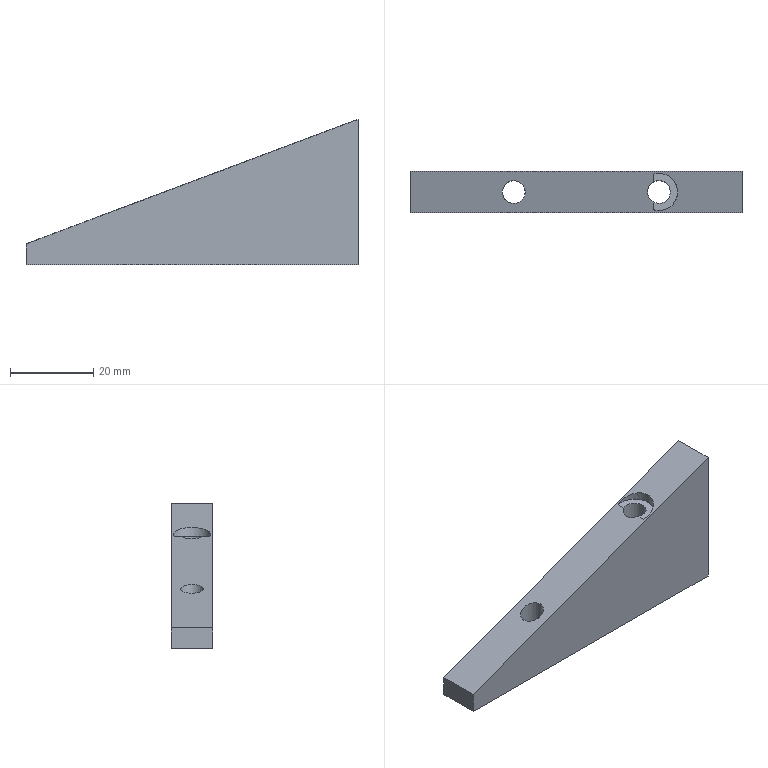NC program | NX | posted with a generic post | part box 80 x 10 x 35 mm
Whole program:
N10 G17 G21 G94 G90
(FACE_MILLING , TOOL : D20)
N12 T00 M6
N14 G54
N16 G17 G0 G90 X60. Y-13.75 B0. C0. S0 M3
N18 G43 Z20. H0
N20 Z4.
N22 G94 G1 Z1. F250.
N24 X50.
N26 X-50.
N28 Y0.
N30 X50.
N32 Y13.75
N34 X-50.
N36 X-60.
N38 Z4.
N40 G0 Z20.
N42 X60. Y-13.75
N44 Z3.
N46 G1 Z0.
N48 X50.
N50 X-50.
N52 Y0.
N54 X50.
N56 Y13.75
N58 X-50.
N60 X-60.
N62 Z3.
N64 G0 Z20.
N66 M5
(PLANAR_PROFILE , TOOL : D10)
N68 T01 M6
N70 G54
N72 G17 G0 G90 X50.15 Y-22.65 B0. C0. S0 M3
N74 G43 Z20. H1
N76 Z0.5
N78 G94 G1 Z-0.5 F250.
N80 X45.15
N82 X-45.15
N84 Y-8.931
N86 X45.15 Y24.931
N88 Y-22.65
N90 Y-27.65
N92 Z0.5
N94 G0 X50.15 Y-22.65 Z0.
N96 G1 Z-1.
N98 X45.15
N100 X-45.15
N102 Y-8.931
N104 X45.15 Y24.931
N106 Y-22.65
N108 Y-27.65
N110 Z0.
N112 G0 X50.15 Y-22.65 Z-0.5
N114 G1 Z-1.5
N116 X45.15
N118 X-45.15
N120 Y-8.931
N122 X45.15 Y24.931
N124 Y-22.65
N126 Y-27.65
N128 Z-0.5
N130 G0 X50.15 Y-22.65 Z-1.
N132 G1 Z-2.
N134 X45.15
N136 X-45.15
N138 Y-8.931
N140 X45.15 Y24.931
N142 Y-22.65
N144 Y-27.65
N146 Z-1.
N148 G0 X50.15 Y-22.65 Z-1.5
N150 G1 Z-2.5
N152 X45.15
N154 X-45.15
N156 Y-8.931
N158 X45.15 Y24.931
N160 Y-22.65
N162 Y-27.65
N164 Z-1.5
N166 G0 X50.15 Y-22.65 Z-2.
N168 G1 Z-3.
N170 X45.15
N172 X-45.15
N174 Y-8.931
N176 X45.15 Y24.931
N178 Y-22.65
N180 Y-27.65
N182 Z-2.
N184 G0 X50.15 Y-22.65 Z-2.5
N186 G1 Z-3.5
N188 X45.15
N190 X-45.15
N192 Y-8.931
N194 X45.15 Y24.931
N196 Y-22.65
N198 Y-27.65
N200 Z-2.5
N202 G0 X50.15 Y-22.65 Z-3.
N204 G1 Z-4.
N206 X45.15
N208 X-45.15
N210 Y-8.931
N212 X45.15 Y24.931
N214 Y-22.65
N216 Y-27.65
N218 Z-3.
N220 G0 X50.15 Y-22.65 Z-3.5
N222 G1 Z-4.5
N224 X45.15
N226 X-45.15
N228 Y-8.931
N230 X45.15 Y24.931
N232 Y-22.65
N234 Y-27.65
N236 Z-3.5
N238 G0 X50.15 Y-22.65 Z-4.
N240 G1 Z-5.
N242 X45.15
N244 X-45.15
N246 Y-8.931
N248 X45.15 Y24.931
N250 Y-22.65
N252 Y-27.65
N254 Z-4.
N256 G0 X50.15 Y-22.65 Z-4.5
N258 G1 Z-5.5
N260 X45.15
N262 X-45.15
N264 Y-8.931
N266 X45.15 Y24.931
N268 Y-22.65
N270 Y-27.65
N272 Z-4.5
N274 G0 X50.15 Y-22.65 Z-5.
N276 G1 Z-6.
N278 X45.15
N280 X-45.15
N282 Y-8.931
N284 X45.15 Y24.931
N286 Y-22.65
N288 Y-27.65
N290 Z-5.
N292 G0 X50.15 Y-22.65 Z-5.5
N294 G1 Z-6.5
N296 X45.15
N298 X-45.15
N300 Y-8.931
N302 X45.15 Y24.931
N304 Y-22.65
N306 Y-27.65
N308 Z-5.5
N310 G0 X50.15 Y-22.65 Z-6.
N312 G1 Z-7.
N314 X45.15
N316 X-45.15
N318 Y-8.931
N320 X45.15 Y24.931
N322 Y-22.65
N324 Y-27.65
N326 Z-6.
N328 G0 X50.15 Y-22.65 Z-6.5
N330 G1 Z-7.5
N332 X45.15
N334 X-45.15
N336 Y-8.931
N338 X45.15 Y24.931
N340 Y-22.65
N342 Y-27.65
N344 Z-6.5
N346 G0 X50.15 Y-22.65 Z-7.
N348 G1 Z-8.
N350 X45.15
N352 X-45.15
N354 Y-8.931
N356 X45.15 Y24.931
N358 Y-22.65
N360 Y-27.65
N362 Z-7.
N364 G0 X50.15 Y-22.65 Z-7.5
N366 G1 Z-8.5
N368 X45.15
N370 X-45.15
N372 Y-8.931
N374 X45.15 Y24.931
N376 Y-22.65
N378 Y-27.65
N380 Z-7.5
N382 G0 X50.15 Y-22.65 Z-8.
N384 G1 Z-9.
N386 X45.15
N388 X-45.15
N390 Y-8.931
N392 X45.15 Y24.931
N394 Y-22.65
N396 Y-27.65
N398 Z-8.
N400 G0 X50.15 Y-22.65 Z-8.5
N402 G1 Z-9.5
N404 X45.15
N406 X-45.15
N408 Y-8.931
N410 X45.15 Y24.931
N412 Y-22.65
N414 Y-27.65
N416 Z-8.5
N418 G0 X50.15 Y-22.65 Z-9.
N420 G1 Z-10.
N422 X45.15
N424 X-45.15
N426 Y-8.931
N428 X45.15 Y24.931
N430 Y-22.65
N432 Y-27.65
N434 Z-9.
N436 G0 Z20.
N438 M5
(PLANAR_MILL , TOOL : D6)
N440 T00 M6
N442 G53
N444 G17 G0 G90 X-24.265 Y-0.247 B0. C0. S0 M3
N446 G43 Z20. H0
N448 Z-4.35
N450 G94 G1 Z-5.35 F250.
N452 X-20.444 Y-1.433
N454 G3 X-20.444 Y1.433 R-1.5
N456 G1 X-24.265 Y0.247
N458 Z-4.35
N460 G0 Z20.
N462 Y-0.247
N464 Z-4.7
N466 G1 Z-5.7
N468 X-20.444 Y-1.433
N470 G3 X-20.444 Y1.433 R-1.5
N472 G1 X-24.265 Y0.247
N474 Z-4.7
N476 G0 Z20.
N478 Y-0.247
N480 Z-5.05
N482 G1 Z-6.05
N484 X-20.444 Y-1.433
N486 G3 X-20.444 Y1.433 R-1.5
N488 G1 X-24.265 Y0.247
N490 Z-5.05
N492 G0 Z20.
N494 Y-0.247
N496 Z-5.4
N498 G1 Z-6.4
N500 X-20.444 Y-1.433
N502 G3 X-20.444 Y1.433 R-1.5
N504 G1 X-24.265 Y0.247
N506 Z-5.4
N508 G0 Z20.
N510 Y-0.247
N512 Z-5.75
N514 G1 Z-6.75
N516 X-20.444 Y-1.433
N518 G3 X-20.444 Y1.433 R-1.5
N520 G1 X-24.265 Y0.247
N522 Z-5.75
N524 G0 Z20.
N526 Y-0.247
N528 Z-6.1
N530 G1 Z-7.1
N532 X-20.444 Y-1.433
N534 G3 X-20.444 Y1.433 R-1.5
N536 G1 X-24.265 Y0.247
N538 Z-6.1
N540 G0 Z20.
N542 Y-0.247
N544 Z-6.45
N546 G1 Z-7.45
N548 X-20.444 Y-1.433
N550 G3 X-20.444 Y1.433 R-1.5
N552 G1 X-24.265 Y0.247
N554 Z-6.45
N556 G0 Z20.
N558 Y-0.247
N560 Z-6.8
N562 G1 Z-7.8
N564 X-20.444 Y-1.433
N566 G3 X-20.444 Y1.433 R-1.5
N568 G1 X-24.265 Y0.247
N570 Z-6.8
N572 G0 Z20.
N574 Y-0.247
N576 Z-7.
N578 G1 Z-8.
N580 X-20.444 Y-1.433
N582 G3 X-20.444 Y1.433 R-1.5
N584 G1 X-24.265 Y0.247
N586 Z-7.
N588 G0 Z20.
N590 M5
(PLANAR_MILL_1 , TOOL : D4)
N592 M6
N594 G53
N596 G17 G0 G90 X-55.426 Y0.065 B0. C0. S0 M3
N598 G43 Z20. H0
N600 Z-20.1
N602 G94 G3 X-55.426 Y0.065 Z-20.298 I0.354 J-0.065 F250.
N604 X-55.43 Y0.041 Z-20.3 R0.36
N606 G1 X-55.435 Y0.
N608 X-55.34 Y-0.27
N610 X-55.121 Y-0.415
N612 X-54.961 Y-0.424
N614 X-54.833 Y-0.393
N616 X-54.61 Y-0.209
N618 X-54.577 Y0.112
N620 G3 X-55.171 Y0.399 R0.454
N622 G1 X-55.39 Y0.194
N624 X-55.422 Y0.106
N626 X-55.435 Y0.
N628 Z-20.1
N630 G0 Z-19.7
N632 X-55.426 Y0.065
N634 Z-20.4
N636 G3 X-55.426 Y0.065 Z-20.598 I0.354 J-0.065
N638 X-55.43 Y0.041 Z-20.6 R0.36
N640 G1 X-55.435 Y0.
N642 X-55.34 Y-0.27
N644 X-55.121 Y-0.415
N646 X-54.961 Y-0.424
N648 X-54.833 Y-0.393
N650 X-54.61 Y-0.209
N652 X-54.577 Y0.112
N654 G3 X-55.171 Y0.399 R0.454
N656 G1 X-55.39 Y0.194
N658 X-55.422 Y0.106
N660 X-55.435 Y0.
N662 Z-20.4
N664 G0 Z-20.
N666 X-55.426 Y0.065
N668 Z-20.7
N670 G3 X-55.426 Y0.065 Z-20.898 I0.354 J-0.065
N672 X-55.43 Y0.041 Z-20.9 R0.36
N674 G1 X-55.435 Y0.
N676 X-55.34 Y-0.27
N678 X-55.121 Y-0.415
N680 X-54.961 Y-0.424
N682 X-54.833 Y-0.393
N684 X-54.61 Y-0.209
N686 X-54.577 Y0.112
N688 G3 X-55.171 Y0.399 R0.454
N690 G1 X-55.39 Y0.194
N692 X-55.422 Y0.106
N694 X-55.435 Y0.
N696 Z-20.7
N698 G0 Z-20.3
N700 X-55.426 Y0.065
N702 Z-21.
N704 G3 X-55.426 Y0.065 Z-21.198 I0.354 J-0.065
N706 X-55.43 Y0.041 Z-21.2 R0.36
N708 G1 X-55.435 Y0.
N710 X-55.34 Y-0.27
N712 X-55.121 Y-0.415
N714 X-54.961 Y-0.424
N716 X-54.833 Y-0.393
N718 X-54.61 Y-0.209
N720 X-54.577 Y0.112
N722 G3 X-55.171 Y0.399 R0.454
N724 G1 X-55.39 Y0.194
N726 X-55.422 Y0.106
N728 X-55.435 Y0.
N730 Z-21.
N732 G0 Z-20.6
N734 X-55.426 Y0.065
N736 Z-21.3
N738 G3 X-55.426 Y0.065 Z-21.498 I0.354 J-0.065
N740 X-55.43 Y0.041 Z-21.5 R0.36
N742 G1 X-55.435 Y0.
N744 X-55.34 Y-0.27
N746 X-55.121 Y-0.415
N748 X-54.961 Y-0.424
N750 X-54.833 Y-0.393
N752 X-54.61 Y-0.209
N754 X-54.577 Y0.112
N756 G3 X-55.171 Y0.399 R0.454
N758 G1 X-55.39 Y0.194
N760 X-55.422 Y0.106
N762 X-55.435 Y0.
N764 Z-21.3
N766 G0 Z-20.9
N768 X-55.426 Y0.065
N770 Z-21.6
N772 G3 X-55.426 Y0.065 Z-21.798 I0.354 J-0.065
N774 X-55.43 Y0.041 Z-21.8 R0.36
N776 G1 X-55.435 Y0.
N778 X-55.34 Y-0.27
N780 X-55.121 Y-0.415
N782 X-54.961 Y-0.424
N784 X-54.833 Y-0.393
N786 X-54.61 Y-0.209
N788 X-54.577 Y0.112
N790 G3 X-55.171 Y0.399 R0.454
N792 G1 X-55.39 Y0.194
N794 X-55.422 Y0.106
N796 X-55.435 Y0.
N798 Z-21.6
N800 G0 Z-21.2
N802 X-55.426 Y0.065
N804 Z-21.8
N806 G3 X-55.426 Y0.065 Z-21.998 I0.354 J-0.065
N808 X-55.43 Y0.041 Z-22. R0.36
N810 G1 X-55.435 Y0.
N812 X-55.34 Y-0.27
N814 X-55.121 Y-0.415
N816 X-54.961 Y-0.424
N818 X-54.833 Y-0.393
N820 X-54.61 Y-0.209
N822 X-54.577 Y0.112
N824 G3 X-55.171 Y0.399 R0.454
N826 G1 X-55.39 Y0.194
N828 X-55.422 Y0.106
N830 X-55.435 Y0.
N832 Z-21.8
N834 G0 Z20.
N836 M5
(PECK_DRILLING , TOOL : DR5.5)
N838 M6
N840 G53
N842 G17 G0 G90 X-20. Y0. B0. C0. S0 M3
N844 G43 Z20. H0
N846 G94 G83 G99 Z-28. F250. Q2.75 R-5.
N848 X-55. Z-39.594 R-16.594
N850 G80
N852 G0 X-55. Y0. Z20.
N854 M5
N856 M2